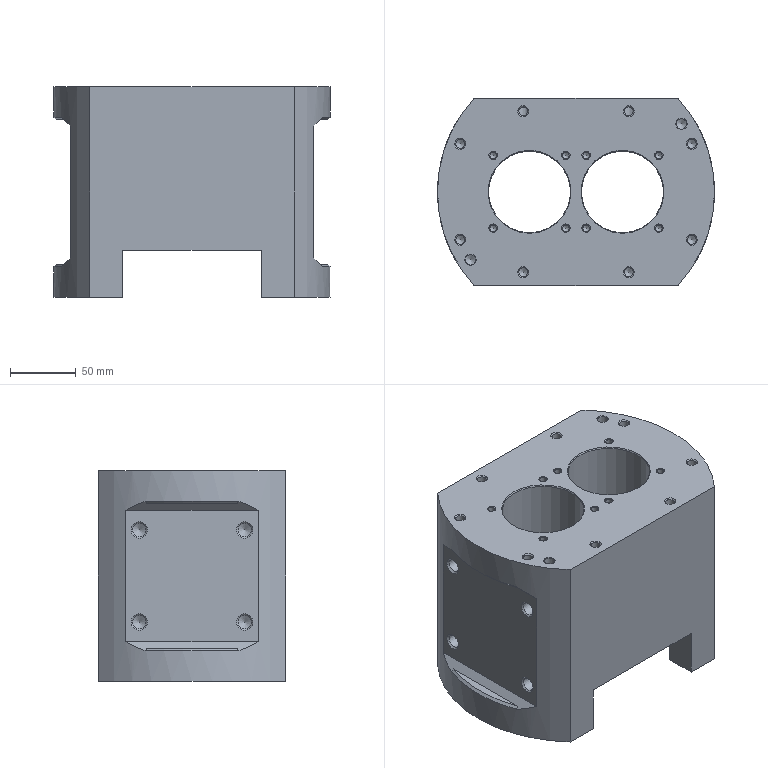Part | 1 solid | 152 faces | box 210 x 142 x 160 mm | volume 2692177 mm3 | cone 86 | cylinder 46 | plane 20 | commonest cylinder face diameters 5 x16 6.8 x8 10.2 x8 8.5 x4 8 x2 10 x2